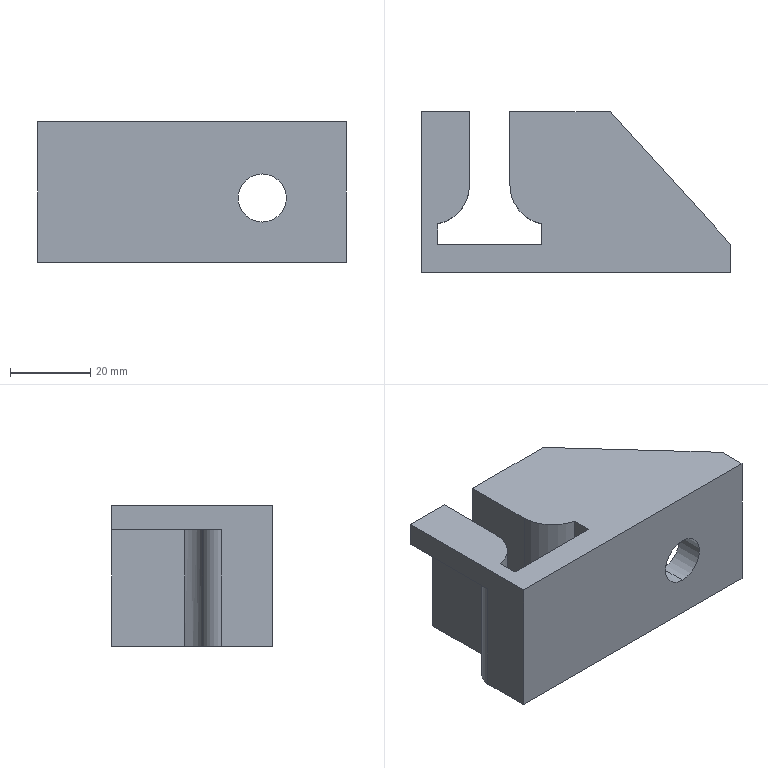Part | SolidWorks | features ICE 4, Fillet 2, MirrorPattern 2, Extrusion 1 | 1 solid | 27 faces | box 77 x 40 x 35 mm | volume 36799 mm3 | plane 19 | cylinder 6 | spline 2 | commonest cylinder face diameters 10 x2 12 x2 20 x2
STEP:
#1=CARTESIAN_POINT('',(39.,0.,-4.638));
#2=VERTEX_POINT('',#1);
#3=CARTESIAN_POINT('',(39.,0.,-16.638));
#4=VERTEX_POINT('',#3);
#5=CARTESIAN_POINT('',(39.,0.,-10.638));
#6=DIRECTION('',(0.,-1.,0.));
#7=DIRECTION('',(0.,0.,1.));
#8=AXIS2_PLACEMENT_3D('',#5,#6,#7);
#9=CIRCLE('',#8,6.);
#10=EDGE_CURVE('',#2,#4,#9,.T.);
#11=ORIENTED_EDGE('',*,*,#10,.T.);
#12=CARTESIAN_POINT('',(39.,7.,-16.638));
#13=VERTEX_POINT('',#12);
#14=CARTESIAN_POINT('',(39.,-3.,-16.638));
#15=DIRECTION('',(0.,1.,0.));
#16=VECTOR('',#15,1000.);
#17=LINE('',#14,#16);
#18=EDGE_CURVE('',#4,#13,#17,.T.);
#19=ORIENTED_EDGE('',*,*,#18,.T.);
#20=CARTESIAN_POINT('',(39.,7.,-4.638));
#21=VERTEX_POINT('',#20);
#22=CARTESIAN_POINT('',(39.,7.,-10.638));
#23=DIRECTION('',(0.,-1.,0.));
#24=DIRECTION('',(0.,0.,1.));
#25=AXIS2_PLACEMENT_3D('',#22,#23,#24);
#26=CIRCLE('',#25,6.);
#27=EDGE_CURVE('',#21,#13,#26,.T.);
#28=ORIENTED_EDGE('',*,*,#27,.F.);
#29=CARTESIAN_POINT('',(39.,-3.,-4.638));
#30=DIRECTION('',(0.,1.,0.));
#31=VECTOR('',#30,1000.);
#32=LINE('',#29,#31);
#33=EDGE_CURVE('',#2,#21,#32,.T.);
#34=ORIENTED_EDGE('',*,*,#33,.F.);
#35=EDGE_LOOP('',(#11,#19,#28,#34));
#36=FACE_OUTER_BOUND('',#35,.T.);
#37=CARTESIAN_POINT('',(39.,-3.,-10.638));
#38=DIRECTION('',(0.,1.,0.));
#39=DIRECTION('',(0.,0.,1.));
#40=AXIS2_PLACEMENT_3D('',#37,#38,#39);
#41=CYLINDRICAL_SURFACE('',#40,6.);
#42=ADVANCED_FACE('',(#36),#41,.F.);
#43=CARTESIAN_POINT('',(17.,7.,-26.638));
#44=VERTEX_POINT('',#43);
#45=CARTESIAN_POINT('',(17.,7.,2.362));
#46=VERTEX_POINT('',#45);
#47=CARTESIAN_POINT('',(17.,7.,-61.752));
#48=DIRECTION('',(0.,0.,1.));
#49=VECTOR('',#48,1000.);
#50=LINE('',#47,#49);
#51=EDGE_CURVE('',#44,#46,#50,.T.);
#52=ORIENTED_EDGE('',*,*,#51,.T.);
#53=CARTESIAN_POINT('',(60.,7.,2.362));
#54=VERTEX_POINT('',#53);
#55=CARTESIAN_POINT('',(13.,7.,2.362));
#56=DIRECTION('',(-1.,0.,0.));
#57=VECTOR('',#56,1000.);
#58=LINE('',#55,#57);
#59=EDGE_CURVE('',#54,#46,#58,.T.);
#60=ORIENTED_EDGE('',*,*,#59,.F.);
#61=CARTESIAN_POINT('',(60.,7.,-26.638));
#62=VERTEX_POINT('',#61);
#63=CARTESIAN_POINT('',(60.,7.,-26.638));
#64=DIRECTION('',(0.,0.,-1.));
#65=VECTOR('',#64,1000.);
#66=LINE('',#63,#65);
#67=EDGE_CURVE('',#54,#62,#66,.T.);
#68=ORIENTED_EDGE('',*,*,#67,.T.);
#69=CARTESIAN_POINT('',(-60.,7.,-26.638));
#70=DIRECTION('',(-1.,0.,0.));
#71=VECTOR('',#70,1000.);
#72=LINE('',#69,#71);
#73=EDGE_CURVE('',#62,#44,#72,.T.);
#74=ORIENTED_EDGE('',*,*,#73,.T.);
#75=EDGE_LOOP('',(#52,#60,#68,#74));
#76=FACE_OUTER_BOUND('',#75,.T.);
#77=ORIENTED_EDGE('',*,*,#27,.T.);
#78=CARTESIAN_POINT('',(39.,7.,-10.638));
#79=DIRECTION('',(0.,-1.,0.));
#80=DIRECTION('',(0.,0.,1.));
#81=AXIS2_PLACEMENT_3D('',#78,#79,#80);
#82=CIRCLE('',#81,6.);
#83=EDGE_CURVE('',#13,#21,#82,.T.);
#84=ORIENTED_EDGE('',*,*,#83,.T.);
#85=EDGE_LOOP('',(#77,#84));
#86=FACE_BOUND('',#85,.T.);
#87=CARTESIAN_POINT('',(0.,7.,0.));
#88=DIRECTION('',(0.,1.,0.));
#89=DIRECTION('',(0.,0.,1.));
#90=AXIS2_PLACEMENT_3D('',#87,#88,#89);
#91=PLANE('',#90);
#92=ADVANCED_FACE('',(#76,#86),#91,.T.);
#93=CARTESIAN_POINT('',(-17.,0.,8.362));
#94=VERTEX_POINT('',#93);
#95=CARTESIAN_POINT('',(60.,0.,8.362));
#96=VERTEX_POINT('',#95);
#97=CARTESIAN_POINT('',(-60.,0.,8.362));
#98=DIRECTION('',(1.,0.,0.));
#99=VECTOR('',#98,1000.);
#100=LINE('',#97,#99);
#101=EDGE_CURVE('',#94,#96,#100,.T.);
#102=ORIENTED_EDGE('',*,*,#101,.F.);
#103=CARTESIAN_POINT('',(-17.,0.,-26.638));
#104=VERTEX_POINT('',#103);
#105=CARTESIAN_POINT('',(-17.,0.,0.));
#106=DIRECTION('',(0.,0.,-1.));
#107=VECTOR('',#106,1000.);
#108=LINE('',#105,#107);
#109=EDGE_CURVE('',#94,#104,#108,.T.);
#110=ORIENTED_EDGE('',*,*,#109,.T.);
#111=CARTESIAN_POINT('',(60.,0.,-26.638));
#112=VERTEX_POINT('',#111);
#113=CARTESIAN_POINT('',(-60.,0.,-26.638));
#114=DIRECTION('',(-1.,0.,0.));
#115=VECTOR('',#114,1000.);
#116=LINE('',#113,#115);
#117=EDGE_CURVE('',#112,#104,#116,.T.);
#118=ORIENTED_EDGE('',*,*,#117,.F.);
#119=CARTESIAN_POINT('',(60.,0.,-26.638));
#120=DIRECTION('',(0.,0.,-1.));
#121=VECTOR('',#120,1000.);
#122=LINE('',#119,#121);
#123=EDGE_CURVE('',#96,#112,#122,.T.);
#124=ORIENTED_EDGE('',*,*,#123,.F.);
#125=EDGE_LOOP('',(#102,#110,#118,#124));
#126=FACE_OUTER_BOUND('',#125,.T.);
#127=ORIENTED_EDGE('',*,*,#10,.F.);
#128=CARTESIAN_POINT('',(39.,0.,-10.638));
#129=DIRECTION('',(0.,-1.,0.));
#130=DIRECTION('',(0.,0.,1.));
#131=AXIS2_PLACEMENT_3D('',#128,#129,#130);
#132=CIRCLE('',#131,6.);
#133=EDGE_CURVE('',#4,#2,#132,.T.);
#134=ORIENTED_EDGE('',*,*,#133,.F.);
#135=EDGE_LOOP('',(#127,#134));
#136=FACE_BOUND('',#135,.T.);
#137=CARTESIAN_POINT('',(0.,0.,0.));
#138=DIRECTION('',(0.,1.,0.));
#139=DIRECTION('',(0.,0.,1.));
#140=AXIS2_PLACEMENT_3D('',#137,#138,#139);
#141=PLANE('',#140);
#142=ADVANCED_FACE('',(#126,#136),#141,.F.);
#143=CARTESIAN_POINT('',(13.,7.,-26.638));
#144=VERTEX_POINT('',#143);
#145=CARTESIAN_POINT('',(13.,7.,8.362));
#146=VERTEX_POINT('',#145);
#147=CARTESIAN_POINT('',(13.,7.,2.362));
#148=DIRECTION('',(0.,0.,1.));
#149=VECTOR('',#148,1000.);
#150=LINE('',#147,#149);
#151=EDGE_CURVE('',#144,#146,#150,.T.);
#152=ORIENTED_EDGE('',*,*,#151,.F.);
#153=CARTESIAN_POINT('',(-13.,7.,-26.638));
#154=VERTEX_POINT('',#153);
#155=CARTESIAN_POINT('',(-60.,7.,-26.638));
#156=DIRECTION('',(-1.,0.,0.));
#157=VECTOR('',#156,1000.);
#158=LINE('',#155,#157);
#159=EDGE_CURVE('',#144,#154,#158,.T.);
#160=ORIENTED_EDGE('',*,*,#159,.T.);
#161=CARTESIAN_POINT('',(-13.,7.,8.362));
#162=VERTEX_POINT('',#161);
#163=CARTESIAN_POINT('',(-13.,7.,2.362));
#164=DIRECTION('',(0.,0.,1.));
#165=VECTOR('',#164,1000.);
#166=LINE('',#163,#165);
#167=EDGE_CURVE('',#154,#162,#166,.T.);
#168=ORIENTED_EDGE('',*,*,#167,.T.);
#169=CARTESIAN_POINT('',(-60.,7.,8.362));
#170=DIRECTION('',(1.,0.,0.));
#171=VECTOR('',#170,1000.);
#172=LINE('',#169,#171);
#173=EDGE_CURVE('',#162,#146,#172,.T.);
#174=ORIENTED_EDGE('',*,*,#173,.T.);
#175=EDGE_LOOP('',(#152,#160,#168,#174));
#176=FACE_OUTER_BOUND('',#175,.T.);
#177=CARTESIAN_POINT('',(0.,7.,0.));
#178=DIRECTION('',(0.,1.,0.));
#179=DIRECTION('',(0.,0.,1.));
#180=AXIS2_PLACEMENT_3D('',#177,#178,#179);
#181=PLANE('',#180);
#182=ADVANCED_FACE('',(#176),#181,.T.);
#183=CARTESIAN_POINT('',(-13.534,17.332,2.362));
#184=VERTEX_POINT('',#183);
#185=CARTESIAN_POINT('',(-17.,12.573,2.362));
#186=VERTEX_POINT('',#185);
#187=CARTESIAN_POINT('',(-12.,12.573,2.362));
#188=DIRECTION('',(0.,0.,1.));
#189=DIRECTION('',(1.,0.,0.));
#190=AXIS2_PLACEMENT_3D('',#187,#188,#189);
#191=CIRCLE('',#190,5.);
#192=EDGE_CURVE('',#184,#186,#191,.T.);
#193=ORIENTED_EDGE('',*,*,#192,.T.);
#194=CARTESIAN_POINT('',(-17.,40.,2.362));
#195=VERTEX_POINT('',#194);
#196=CARTESIAN_POINT('',(-17.,0.,2.362));
#197=DIRECTION('',(0.,1.,0.));
#198=VECTOR('',#197,1000.);
#199=LINE('',#196,#198);
#200=EDGE_CURVE('',#186,#195,#199,.T.);
#201=ORIENTED_EDGE('',*,*,#200,.T.);
#202=CARTESIAN_POINT('',(-9.,40.,2.362));
#203=VERTEX_POINT('',#202);
#204=CARTESIAN_POINT('',(-30.,40.,2.362));
#205=DIRECTION('',(-1.,0.,0.));
#206=VECTOR('',#205,1000.);
#207=LINE('',#204,#206);
#208=EDGE_CURVE('',#203,#195,#207,.T.);
#209=ORIENTED_EDGE('',*,*,#208,.F.);
#210=CARTESIAN_POINT('',(-9.,21.798,2.362));
#211=VERTEX_POINT('',#210);
#212=CARTESIAN_POINT('',(-9.,21.798,2.362));
#213=DIRECTION('',(0.,1.,0.));
#214=VECTOR('',#213,1000.);
#215=LINE('',#212,#214);
#216=EDGE_CURVE('',#211,#203,#215,.T.);
#217=ORIENTED_EDGE('',*,*,#216,.F.);
#218=CARTESIAN_POINT('',(-13.534,17.332,2.362));
#219=CARTESIAN_POINT('',(-10.568,18.288,2.362));
#220=CARTESIAN_POINT('',(-9.,21.798,2.362));
#221=B_SPLINE_CURVE_WITH_KNOTS('',2,(#218,#219,#220),.UNSPECIFIED.,.F.,.F.,(3,3),(0.3423,1.),.UNSPECIFIED.);
#222=EDGE_CURVE('',#184,#211,#221,.T.);
#223=ORIENTED_EDGE('',*,*,#222,.F.);
#224=EDGE_LOOP('',(#193,#201,#209,#217,#223));
#225=FACE_OUTER_BOUND('',#224,.T.);
#226=CARTESIAN_POINT('',(0.,0.,2.362));
#227=DIRECTION('',(0.,0.,1.));
#228=DIRECTION('',(1.,0.,0.));
#229=AXIS2_PLACEMENT_3D('',#226,#227,#228);
#230=PLANE('',#229);
#231=ADVANCED_FACE('',(#225),#230,.F.);
#232=CARTESIAN_POINT('',(-5.,40.,8.362));
#233=VERTEX_POINT('',#232);
#234=CARTESIAN_POINT('',(-17.,40.,8.362));
#235=VERTEX_POINT('',#234);
#236=CARTESIAN_POINT('',(-30.,40.,8.362));
#237=DIRECTION('',(-1.,0.,0.));
#238=VECTOR('',#237,1000.);
#239=LINE('',#236,#238);
#240=EDGE_CURVE('',#233,#235,#239,.T.);
#241=ORIENTED_EDGE('',*,*,#240,.T.);
#242=CARTESIAN_POINT('',(-17.,7.,8.362));
#243=DIRECTION('',(0.,-1.,0.));
#244=VECTOR('',#243,1000.);
#245=LINE('',#242,#244);
#246=EDGE_CURVE('',#235,#94,#245,.T.);
#247=ORIENTED_EDGE('',*,*,#246,.T.);
#248=ORIENTED_EDGE('',*,*,#101,.T.);
#249=CARTESIAN_POINT('',(60.,7.,8.362));
#250=VERTEX_POINT('',#249);
#251=CARTESIAN_POINT('',(60.,7.,8.362));
#252=DIRECTION('',(0.,-1.,0.));
#253=VECTOR('',#252,1000.);
#254=LINE('',#251,#253);
#255=EDGE_CURVE('',#250,#96,#254,.T.);
#256=ORIENTED_EDGE('',*,*,#255,.F.);
#257=CARTESIAN_POINT('',(30.,40.,8.362));
#258=VERTEX_POINT('',#257);
#259=CARTESIAN_POINT('',(60.,7.,8.362));
#260=DIRECTION('',(0.6727,-0.7399,0.));
#261=VECTOR('',#260,1000.);
#262=LINE('',#259,#261);
#263=EDGE_CURVE('',#258,#250,#262,.T.);
#264=ORIENTED_EDGE('',*,*,#263,.F.);
#265=CARTESIAN_POINT('',(5.,40.,8.362));
#266=VERTEX_POINT('',#265);
#267=CARTESIAN_POINT('',(30.,40.,8.362));
#268=DIRECTION('',(1.,0.,0.));
#269=VECTOR('',#268,1000.);
#270=LINE('',#267,#269);
#271=EDGE_CURVE('',#266,#258,#270,.T.);
#272=ORIENTED_EDGE('',*,*,#271,.F.);
#273=CARTESIAN_POINT('',(5.,21.798,8.362));
#274=VERTEX_POINT('',#273);
#275=CARTESIAN_POINT('',(5.,40.,8.362));
#276=DIRECTION('',(0.,1.,0.));
#277=VECTOR('',#276,1000.);
#278=LINE('',#275,#277);
#279=EDGE_CURVE('',#274,#266,#278,.T.);
#280=ORIENTED_EDGE('',*,*,#279,.F.);
#281=CARTESIAN_POINT('',(13.,12.,8.362));
#282=VERTEX_POINT('',#281);
#283=CARTESIAN_POINT('',(15.,21.798,8.362));
#284=DIRECTION('',(0.,0.,1.));
#285=DIRECTION('',(-1.,0.,0.));
#286=AXIS2_PLACEMENT_3D('',#283,#284,#285);
#287=CIRCLE('',#286,10.);
#288=EDGE_CURVE('',#274,#282,#287,.T.);
#289=ORIENTED_EDGE('',*,*,#288,.T.);
#290=CARTESIAN_POINT('',(13.,12.,8.362));
#291=DIRECTION('',(0.,1.,0.));
#292=VECTOR('',#291,1000.);
#293=LINE('',#290,#292);
#294=EDGE_CURVE('',#146,#282,#293,.T.);
#295=ORIENTED_EDGE('',*,*,#294,.F.);
#296=ORIENTED_EDGE('',*,*,#173,.F.);
#297=CARTESIAN_POINT('',(-13.,12.,8.362));
#298=VERTEX_POINT('',#297);
#299=CARTESIAN_POINT('',(-13.,12.,8.362));
#300=DIRECTION('',(0.,1.,0.));
#301=VECTOR('',#300,1000.);
#302=LINE('',#299,#301);
#303=EDGE_CURVE('',#162,#298,#302,.T.);
#304=ORIENTED_EDGE('',*,*,#303,.T.);
#305=CARTESIAN_POINT('',(-5.,21.798,8.362));
#306=VERTEX_POINT('',#305);
#307=CARTESIAN_POINT('',(-15.,21.798,8.362));
#308=DIRECTION('',(0.,0.,1.));
#309=DIRECTION('',(-1.,0.,0.));
#310=AXIS2_PLACEMENT_3D('',#307,#308,#309);
#311=CIRCLE('',#310,10.);
#312=EDGE_CURVE('',#298,#306,#311,.T.);
#313=ORIENTED_EDGE('',*,*,#312,.T.);
#314=CARTESIAN_POINT('',(-5.,40.,8.362));
#315=DIRECTION('',(0.,1.,0.));
#316=VECTOR('',#315,1000.);
#317=LINE('',#314,#316);
#318=EDGE_CURVE('',#306,#233,#317,.T.);
#319=ORIENTED_EDGE('',*,*,#318,.T.);
#320=EDGE_LOOP('',(#241,#247,#248,#256,#264,#272,#280,#289,#295,#296,#304,#313,#319));
#321=FACE_OUTER_BOUND('',#320,.T.);
#322=CARTESIAN_POINT('',(-60.,7.,8.362));
#323=DIRECTION('',(0.,0.,-1.));
#324=DIRECTION('',(-1.,0.,0.));
#325=AXIS2_PLACEMENT_3D('',#322,#323,#324);
#326=PLANE('',#325);
#327=ADVANCED_FACE('',(#321),#326,.F.);
#328=ORIENTED_EDGE('',*,*,#123,.T.);
#329=CARTESIAN_POINT('',(60.,7.,-26.638));
#330=DIRECTION('',(0.,-1.,0.));
#331=VECTOR('',#330,1000.);
#332=LINE('',#329,#331);
#333=EDGE_CURVE('',#62,#112,#332,.T.);
#334=ORIENTED_EDGE('',*,*,#333,.F.);
#335=ORIENTED_EDGE('',*,*,#67,.F.);
#336=CARTESIAN_POINT('',(60.,7.,-26.638));
#337=DIRECTION('',(0.,0.,-1.));
#338=VECTOR('',#337,1000.);
#339=LINE('',#336,#338);
#340=EDGE_CURVE('',#250,#54,#339,.T.);
#341=ORIENTED_EDGE('',*,*,#340,.F.);
#342=ORIENTED_EDGE('',*,*,#255,.T.);
#343=EDGE_LOOP('',(#328,#334,#335,#341,#342));
#344=FACE_OUTER_BOUND('',#343,.T.);
#345=CARTESIAN_POINT('',(60.,7.,-26.638));
#346=DIRECTION('',(-1.,0.,0.));
#347=DIRECTION('',(0.,0.,1.));
#348=AXIS2_PLACEMENT_3D('',#345,#346,#347);
#349=PLANE('',#348);
#350=ADVANCED_FACE('',(#344),#349,.F.);
#351=ORIENTED_EDGE('',*,*,#117,.T.);
#352=CARTESIAN_POINT('',(-17.,12.573,-26.638));
#353=VERTEX_POINT('',#352);
#354=CARTESIAN_POINT('',(-17.,15.,-26.638));
#355=DIRECTION('',(0.,-1.,0.));
#356=VECTOR('',#355,1000.);
#357=LINE('',#354,#356);
#358=EDGE_CURVE('',#353,#104,#357,.T.);
#359=ORIENTED_EDGE('',*,*,#358,.F.);
#360=CARTESIAN_POINT('',(-13.534,17.332,-26.638));
#361=VERTEX_POINT('',#360);
#362=CARTESIAN_POINT('',(-12.,12.573,-26.638));
#363=DIRECTION('',(0.,0.,-1.));
#364=DIRECTION('',(1.,0.,0.));
#365=AXIS2_PLACEMENT_3D('',#362,#363,#364);
#366=CIRCLE('',#365,5.);
#367=EDGE_CURVE('',#353,#361,#366,.T.);
#368=ORIENTED_EDGE('',*,*,#367,.T.);
#369=CARTESIAN_POINT('',(-9.,21.798,-26.638));
#370=VERTEX_POINT('',#369);
#371=CARTESIAN_POINT('',(-9.,21.798,-26.638));
#372=CARTESIAN_POINT('',(-10.568,18.288,-26.638));
#373=CARTESIAN_POINT('',(-13.534,17.332,-26.638));
#374=B_SPLINE_CURVE_WITH_KNOTS('',2,(#371,#372,#373),.UNSPECIFIED.,.F.,.F.,(3,3),(0.,0.6577),.UNSPECIFIED.);
#375=EDGE_CURVE('',#370,#361,#374,.T.);
#376=ORIENTED_EDGE('',*,*,#375,.F.);
#377=CARTESIAN_POINT('',(-9.,40.,-26.638));
#378=VERTEX_POINT('',#377);
#379=CARTESIAN_POINT('',(-9.,21.798,-26.638));
#380=DIRECTION('',(0.,-1.,0.));
#381=VECTOR('',#380,1000.);
#382=LINE('',#379,#381);
#383=EDGE_CURVE('',#378,#370,#382,.T.);
#384=ORIENTED_EDGE('',*,*,#383,.F.);
#385=CARTESIAN_POINT('',(-5.,40.,-26.638));
#386=VERTEX_POINT('',#385);
#387=CARTESIAN_POINT('',(-5.,40.,-26.638));
#388=DIRECTION('',(-1.,0.,0.));
#389=VECTOR('',#388,1000.);
#390=LINE('',#387,#389);
#391=EDGE_CURVE('',#386,#378,#390,.T.);
#392=ORIENTED_EDGE('',*,*,#391,.F.);
#393=CARTESIAN_POINT('',(-5.,21.798,-26.638));
#394=VERTEX_POINT('',#393);
#395=CARTESIAN_POINT('',(-5.,21.798,-26.638));
#396=DIRECTION('',(0.,1.,0.));
#397=VECTOR('',#396,1000.);
#398=LINE('',#395,#397);
#399=EDGE_CURVE('',#394,#386,#398,.T.);
#400=ORIENTED_EDGE('',*,*,#399,.F.);
#401=CARTESIAN_POINT('',(-13.,12.,-26.638));
#402=VERTEX_POINT('',#401);
#403=CARTESIAN_POINT('',(-15.,21.798,-26.638));
#404=DIRECTION('',(0.,0.,1.));
#405=DIRECTION('',(1.,0.,0.));
#406=AXIS2_PLACEMENT_3D('',#403,#404,#405);
#407=CIRCLE('',#406,10.);
#408=EDGE_CURVE('',#402,#394,#407,.T.);
#409=ORIENTED_EDGE('',*,*,#408,.F.);
#410=CARTESIAN_POINT('',(-13.,7.,-26.638));
#411=DIRECTION('',(0.,1.,0.));
#412=VECTOR('',#411,1000.);
#413=LINE('',#410,#412);
#414=EDGE_CURVE('',#154,#402,#413,.T.);
#415=ORIENTED_EDGE('',*,*,#414,.F.);
#416=ORIENTED_EDGE('',*,*,#159,.F.);
#417=CARTESIAN_POINT('',(13.,12.,-26.638));
#418=VERTEX_POINT('',#417);
#419=CARTESIAN_POINT('',(13.,7.,-26.638));
#420=DIRECTION('',(0.,1.,0.));
#421=VECTOR('',#420,1000.);
#422=LINE('',#419,#421);
#423=EDGE_CURVE('',#144,#418,#422,.T.);
#424=ORIENTED_EDGE('',*,*,#423,.T.);
#425=CARTESIAN_POINT('',(5.,21.798,-26.638));
#426=VERTEX_POINT('',#425);
#427=CARTESIAN_POINT('',(15.,21.798,-26.638));
#428=DIRECTION('',(0.,0.,-1.));
#429=DIRECTION('',(1.,0.,0.));
#430=AXIS2_PLACEMENT_3D('',#427,#428,#429);
#431=CIRCLE('',#430,10.);
#432=EDGE_CURVE('',#418,#426,#431,.T.);
#433=ORIENTED_EDGE('',*,*,#432,.T.);
#434=CARTESIAN_POINT('',(5.,40.,-26.638));
#435=VERTEX_POINT('',#434);
#436=CARTESIAN_POINT('',(5.,21.798,-26.638));
#437=DIRECTION('',(0.,1.,0.));
#438=VECTOR('',#437,1000.);
#439=LINE('',#436,#438);
#440=EDGE_CURVE('',#426,#435,#439,.T.);
#441=ORIENTED_EDGE('',*,*,#440,.T.);
#442=CARTESIAN_POINT('',(9.,40.,-26.638));
#443=VERTEX_POINT('',#442);
#444=CARTESIAN_POINT('',(5.,40.,-26.638));
#445=DIRECTION('',(1.,0.,0.));
#446=VECTOR('',#445,1000.);
#447=LINE('',#444,#446);
#448=EDGE_CURVE('',#435,#443,#447,.T.);
#449=ORIENTED_EDGE('',*,*,#448,.T.);
#450=CARTESIAN_POINT('',(9.,21.798,-26.638));
#451=VERTEX_POINT('',#450);
#452=CARTESIAN_POINT('',(9.,21.798,-26.638));
#453=DIRECTION('',(0.,-1.,0.));
#454=VECTOR('',#453,1000.);
#455=LINE('',#452,#454);
#456=EDGE_CURVE('',#443,#451,#455,.T.);
#457=ORIENTED_EDGE('',*,*,#456,.T.);
#458=CARTESIAN_POINT('',(13.534,17.332,-26.638));
#459=VERTEX_POINT('',#458);
#460=CARTESIAN_POINT('',(9.,21.798,-26.638));
#461=CARTESIAN_POINT('',(10.568,18.288,-26.638));
#462=CARTESIAN_POINT('',(13.534,17.332,-26.638));
#463=B_SPLINE_CURVE_WITH_KNOTS('',2,(#460,#461,#462),.UNSPECIFIED.,.F.,.F.,(3,3),(0.,0.6577),.UNSPECIFIED.);
#464=EDGE_CURVE('',#451,#459,#463,.T.);
#465=ORIENTED_EDGE('',*,*,#464,.T.);
#466=CARTESIAN_POINT('',(17.,12.573,-26.638));
#467=VERTEX_POINT('',#466);
#468=CARTESIAN_POINT('',(12.,12.573,-26.638));
#469=DIRECTION('',(0.,0.,-1.));
#470=DIRECTION('',(1.,0.,0.));
#471=AXIS2_PLACEMENT_3D('',#468,#469,#470);
#472=CIRCLE('',#471,5.);
#473=EDGE_CURVE('',#459,#467,#472,.T.);
#474=ORIENTED_EDGE('',*,*,#473,.T.);
#475=CARTESIAN_POINT('',(17.,7.,-26.638));
#476=DIRECTION('',(0.,-1.,0.));
#477=VECTOR('',#476,1000.);
#478=LINE('',#475,#477);
#479=EDGE_CURVE('',#467,#44,#478,.T.);
#480=ORIENTED_EDGE('',*,*,#479,.T.);
#481=ORIENTED_EDGE('',*,*,#73,.F.);
#482=ORIENTED_EDGE('',*,*,#333,.T.);
#483=EDGE_LOOP('',(#351,#359,#368,#376,#384,#392,#400,#409,#415,#416,#424,#433,#441,#449,#457,#465,#474,#480,#481,#482));
#484=FACE_OUTER_BOUND('',#483,.T.);
#485=CARTESIAN_POINT('',(-60.,7.,-26.638));
#486=DIRECTION('',(0.,0.,1.));
#487=DIRECTION('',(1.,0.,0.));
#488=AXIS2_PLACEMENT_3D('',#485,#486,#487);
#489=PLANE('',#488);
#490=ADVANCED_FACE('',(#484),#489,.F.);
#491=CARTESIAN_POINT('',(-17.,40.,2.362));
#492=DIRECTION('',(0.,0.,-1.));
#493=VECTOR('',#492,1000.);
#494=LINE('',#491,#493);
#495=EDGE_CURVE('',#235,#195,#494,.T.);
#496=ORIENTED_EDGE('',*,*,#495,.F.);
#497=ORIENTED_EDGE('',*,*,#240,.F.);
#498=CARTESIAN_POINT('',(-5.,40.,2.362));
#499=DIRECTION('',(0.,0.,1.));
#500=VECTOR('',#499,1000.);
#501=LINE('',#498,#500);
#502=EDGE_CURVE('',#386,#233,#501,.T.);
#503=ORIENTED_EDGE('',*,*,#502,.F.);
#504=ORIENTED_EDGE('',*,*,#391,.T.);
#505=CARTESIAN_POINT('',(-9.,40.,-61.752));
#506=DIRECTION('',(0.,0.,1.));
#507=VECTOR('',#506,1000.);
#508=LINE('',#505,#507);
#509=EDGE_CURVE('',#378,#203,#508,.T.);
#510=ORIENTED_EDGE('',*,*,#509,.T.);
#511=ORIENTED_EDGE('',*,*,#208,.T.);
#512=EDGE_LOOP('',(#496,#497,#503,#504,#510,#511));
#513=FACE_OUTER_BOUND('',#512,.T.);
#514=CARTESIAN_POINT('',(-30.,40.,2.362));
#515=DIRECTION('',(0.,1.,0.));
#516=DIRECTION('',(-1.,0.,0.));
#517=AXIS2_PLACEMENT_3D('',#514,#515,#516);
#518=PLANE('',#517);
#519=ADVANCED_FACE('',(#513),#518,.T.);
#520=ORIENTED_EDGE('',*,*,#318,.F.);
#521=CARTESIAN_POINT('',(-5.,21.798,2.362));
#522=DIRECTION('',(0.,0.,-1.));
#523=VECTOR('',#522,1000.);
#524=LINE('',#521,#523);
#525=EDGE_CURVE('',#306,#394,#524,.T.);
#526=ORIENTED_EDGE('',*,*,#525,.T.);
#527=ORIENTED_EDGE('',*,*,#399,.T.);
#528=ORIENTED_EDGE('',*,*,#502,.T.);
#529=EDGE_LOOP('',(#520,#526,#527,#528));
#530=FACE_OUTER_BOUND('',#529,.T.);
#531=CARTESIAN_POINT('',(-5.,40.,2.362));
#532=DIRECTION('',(1.,0.,0.));
#533=DIRECTION('',(0.,1.,0.));
#534=AXIS2_PLACEMENT_3D('',#531,#532,#533);
#535=PLANE('',#534);
#536=ADVANCED_FACE('',(#530),#535,.T.);
#537=ORIENTED_EDGE('',*,*,#303,.F.);
#538=ORIENTED_EDGE('',*,*,#167,.F.);
#539=ORIENTED_EDGE('',*,*,#414,.T.);
#540=CARTESIAN_POINT('',(-13.,12.,2.362));
#541=DIRECTION('',(0.,0.,1.));
#542=VECTOR('',#541,1000.);
#543=LINE('',#540,#542);
#544=EDGE_CURVE('',#402,#298,#543,.T.);
#545=ORIENTED_EDGE('',*,*,#544,.T.);
#546=EDGE_LOOP('',(#537,#538,#539,#545));
#547=FACE_OUTER_BOUND('',#546,.T.);
#548=CARTESIAN_POINT('',(-13.,12.,2.362));
#549=DIRECTION('',(1.,0.,0.));
#550=DIRECTION('',(0.,1.,0.));
#551=AXIS2_PLACEMENT_3D('',#548,#549,#550);
#552=PLANE('',#551);
#553=ADVANCED_FACE('',(#547),#552,.T.);
#554=ORIENTED_EDGE('',*,*,#544,.F.);
#555=ORIENTED_EDGE('',*,*,#408,.T.);
#556=ORIENTED_EDGE('',*,*,#525,.F.);
#557=ORIENTED_EDGE('',*,*,#312,.F.);
#558=EDGE_LOOP('',(#554,#555,#556,#557));
#559=FACE_OUTER_BOUND('',#558,.T.);
#560=CARTESIAN_POINT('',(-15.,21.798,2.362));
#561=DIRECTION('',(0.,0.,1.));
#562=DIRECTION('',(1.,0.,0.));
#563=AXIS2_PLACEMENT_3D('',#560,#561,#562);
#564=CYLINDRICAL_SURFACE('',#563,10.);
#565=ADVANCED_FACE('',(#559),#564,.T.);
#566=ORIENTED_EDGE('',*,*,#509,.F.);
#567=ORIENTED_EDGE('',*,*,#383,.T.);
#568=CARTESIAN_POINT('',(-9.,21.798,-61.752));
#569=DIRECTION('',(0.,0.,1.));
#570=VECTOR('',#569,1000.);
#571=LINE('',#568,#570);
#572=EDGE_CURVE('',#370,#211,#571,.T.);
#573=ORIENTED_EDGE('',*,*,#572,.T.);
#574=ORIENTED_EDGE('',*,*,#216,.T.);
#575=EDGE_LOOP('',(#566,#567,#573,#574));
#576=FACE_OUTER_BOUND('',#575,.T.);
#577=CARTESIAN_POINT('',(-9.,21.798,-61.752));
#578=DIRECTION('',(1.,0.,0.));
#579=DIRECTION('',(0.,0.,-1.));
#580=AXIS2_PLACEMENT_3D('',#577,#578,#579);
#581=PLANE('',#580);
#582=ADVANCED_FACE('',(#576),#581,.F.);
#583=ORIENTED_EDGE('',*,*,#375,.T.);
#584=CARTESIAN_POINT('',(-13.534,17.332,-26.638));
#585=DIRECTION('',(0.,0.,1.));
#586=VECTOR('',#585,1000.);
#587=LINE('',#584,#586);
#588=EDGE_CURVE('',#361,#184,#587,.T.);
#589=ORIENTED_EDGE('',*,*,#588,.T.);
#590=ORIENTED_EDGE('',*,*,#222,.T.);
#591=ORIENTED_EDGE('',*,*,#572,.F.);
#592=EDGE_LOOP('',(#583,#589,#590,#591));
#593=FACE_OUTER_BOUND('',#592,.T.);
#594=CARTESIAN_POINT('',(-13.534,17.332,-26.638));
#595=CARTESIAN_POINT('',(-13.534,17.332,2.362));
#596=CARTESIAN_POINT('',(-10.568,18.288,-26.638));
#597=CARTESIAN_POINT('',(-10.568,18.288,2.362));
#598=CARTESIAN_POINT('',(-9.,21.798,-26.638));
#599=CARTESIAN_POINT('',(-9.,21.798,2.362));
#600=B_SPLINE_SURFACE_WITH_KNOTS('',2,1,((#594,#595),(#596,#597),(#598,#599)),.UNSPECIFIED.,.F.,.F.,.F.,(3,3),(2,2),(0.3423,1.),(0.,1.),.UNSPECIFIED.);
#601=ADVANCED_FACE('',(#593),#600,.F.);
#602=ORIENTED_EDGE('',*,*,#358,.T.);
#603=ORIENTED_EDGE('',*,*,#109,.F.);
#604=ORIENTED_EDGE('',*,*,#246,.F.);
#605=ORIENTED_EDGE('',*,*,#495,.T.);
#606=ORIENTED_EDGE('',*,*,#200,.F.);
#607=CARTESIAN_POINT('',(-17.,12.573,-61.752));
#608=DIRECTION('',(0.,0.,-1.));
#609=VECTOR('',#608,1000.);
#610=LINE('',#607,#609);
#611=EDGE_CURVE('',#186,#353,#610,.T.);
#612=ORIENTED_EDGE('',*,*,#611,.T.);
#613=EDGE_LOOP('',(#602,#603,#604,#605,#606,#612));
#614=FACE_OUTER_BOUND('',#613,.T.);
#615=CARTESIAN_POINT('',(-17.,15.,-61.752));
#616=DIRECTION('',(1.,0.,0.));
#617=DIRECTION('',(0.,0.,-1.));
#618=AXIS2_PLACEMENT_3D('',#615,#616,#617);
#619=PLANE('',#618);
#620=ADVANCED_FACE('',(#614),#619,.F.);
#621=ORIENTED_EDGE('',*,*,#294,.T.);
#622=CARTESIAN_POINT('',(13.,12.,2.362));
#623=DIRECTION('',(0.,0.,1.));
#624=VECTOR('',#623,1000.);
#625=LINE('',#622,#624);
#626=EDGE_CURVE('',#418,#282,#625,.T.);
#627=ORIENTED_EDGE('',*,*,#626,.F.);
#628=ORIENTED_EDGE('',*,*,#423,.F.);
#629=ORIENTED_EDGE('',*,*,#151,.T.);
#630=EDGE_LOOP('',(#621,#627,#628,#629));
#631=FACE_OUTER_BOUND('',#630,.T.);
#632=CARTESIAN_POINT('',(13.,12.,2.362));
#633=DIRECTION('',(1.,0.,0.));
#634=DIRECTION('',(0.,1.,0.));
#635=AXIS2_PLACEMENT_3D('',#632,#633,#634);
#636=PLANE('',#635);
#637=ADVANCED_FACE('',(#631),#636,.F.);
#638=CARTESIAN_POINT('',(5.,40.,2.362));
#639=DIRECTION('',(0.,0.,1.));
#640=VECTOR('',#639,1000.);
#641=LINE('',#638,#640);
#642=EDGE_CURVE('',#435,#266,#641,.T.);
#643=ORIENTED_EDGE('',*,*,#642,.F.);
#644=ORIENTED_EDGE('',*,*,#440,.F.);
#645=CARTESIAN_POINT('',(5.,21.798,2.362));
#646=DIRECTION('',(0.,0.,1.));
#647=VECTOR('',#646,1000.);
#648=LINE('',#645,#647);
#649=EDGE_CURVE('',#426,#274,#648,.T.);
#650=ORIENTED_EDGE('',*,*,#649,.T.);
#651=ORIENTED_EDGE('',*,*,#279,.T.);
#652=EDGE_LOOP('',(#643,#644,#650,#651));
#653=FACE_OUTER_BOUND('',#652,.T.);
#654=CARTESIAN_POINT('',(5.,40.,2.362));
#655=DIRECTION('',(1.,0.,0.));
#656=DIRECTION('',(0.,1.,0.));
#657=AXIS2_PLACEMENT_3D('',#654,#655,#656);
#658=PLANE('',#657);
#659=ADVANCED_FACE('',(#653),#658,.F.);
#660=ORIENTED_EDGE('',*,*,#271,.T.);
#661=CARTESIAN_POINT('',(30.,40.,2.362));
#662=VERTEX_POINT('',#661);
#663=CARTESIAN_POINT('',(30.,40.,2.362));
#664=DIRECTION('',(0.,0.,1.));
#665=VECTOR('',#664,1000.);
#666=LINE('',#663,#665);
#667=EDGE_CURVE('',#662,#258,#666,.T.);
#668=ORIENTED_EDGE('',*,*,#667,.F.);
#669=CARTESIAN_POINT('',(9.,40.,2.362));
#670=VERTEX_POINT('',#669);
#671=CARTESIAN_POINT('',(30.,40.,2.362));
#672=DIRECTION('',(1.,0.,0.));
#673=VECTOR('',#672,1000.);
#674=LINE('',#671,#673);
#675=EDGE_CURVE('',#670,#662,#674,.T.);
#676=ORIENTED_EDGE('',*,*,#675,.F.);
#677=CARTESIAN_POINT('',(9.,40.,-61.752));
#678=DIRECTION('',(0.,0.,1.));
#679=VECTOR('',#678,1000.);
#680=LINE('',#677,#679);
#681=EDGE_CURVE('',#443,#670,#680,.T.);
#682=ORIENTED_EDGE('',*,*,#681,.F.);
#683=ORIENTED_EDGE('',*,*,#448,.F.);
#684=ORIENTED_EDGE('',*,*,#642,.T.);
#685=EDGE_LOOP('',(#660,#668,#676,#682,#683,#684));
#686=FACE_OUTER_BOUND('',#685,.T.);
#687=CARTESIAN_POINT('',(30.,40.,2.362));
#688=DIRECTION('',(0.,-1.,0.));
#689=DIRECTION('',(1.,0.,0.));
#690=AXIS2_PLACEMENT_3D('',#687,#688,#689);
#691=PLANE('',#690);
#692=ADVANCED_FACE('',(#686),#691,.F.);
#693=ORIENTED_EDGE('',*,*,#263,.T.);
#694=ORIENTED_EDGE('',*,*,#340,.T.);
#695=CARTESIAN_POINT('',(60.,7.,2.362));
#696=DIRECTION('',(0.6727,-0.7399,0.));
#697=VECTOR('',#696,1000.);
#698=LINE('',#695,#697);
#699=EDGE_CURVE('',#662,#54,#698,.T.);
#700=ORIENTED_EDGE('',*,*,#699,.F.);
#701=ORIENTED_EDGE('',*,*,#667,.T.);
#702=EDGE_LOOP('',(#693,#694,#700,#701));
#703=FACE_OUTER_BOUND('',#702,.T.);
#704=CARTESIAN_POINT('',(60.,7.,2.362));
#705=DIRECTION('',(-0.7399,-0.6727,0.));
#706=DIRECTION('',(0.6727,-0.7399,0.));
#707=AXIS2_PLACEMENT_3D('',#704,#705,#706);
#708=PLANE('',#707);
#709=ADVANCED_FACE('',(#703),#708,.F.);
#710=CARTESIAN_POINT('',(17.,12.573,2.362));
#711=VERTEX_POINT('',#710);
#712=CARTESIAN_POINT('',(17.,7.,2.362));
#713=DIRECTION('',(0.,1.,0.));
#714=VECTOR('',#713,1000.);
#715=LINE('',#712,#714);
#716=EDGE_CURVE('',#46,#711,#715,.T.);
#717=ORIENTED_EDGE('',*,*,#716,.T.);
#718=CARTESIAN_POINT('',(13.534,17.332,2.362));
#719=VERTEX_POINT('',#718);
#720=CARTESIAN_POINT('',(12.,12.573,2.362));
#721=DIRECTION('',(0.,0.,1.));
#722=DIRECTION('',(1.,0.,0.));
#723=AXIS2_PLACEMENT_3D('',#720,#721,#722);
#724=CIRCLE('',#723,5.);
#725=EDGE_CURVE('',#711,#719,#724,.T.);
#726=ORIENTED_EDGE('',*,*,#725,.T.);
#727=CARTESIAN_POINT('',(9.,21.798,2.362));
#728=VERTEX_POINT('',#727);
#729=CARTESIAN_POINT('',(13.534,17.332,2.362));
#730=CARTESIAN_POINT('',(10.568,18.288,2.362));
#731=CARTESIAN_POINT('',(9.,21.798,2.362));
#732=B_SPLINE_CURVE_WITH_KNOTS('',2,(#729,#730,#731),.UNSPECIFIED.,.F.,.F.,(3,3),(0.3423,1.),.UNSPECIFIED.);
#733=EDGE_CURVE('',#719,#728,#732,.T.);
#734=ORIENTED_EDGE('',*,*,#733,.T.);
#735=CARTESIAN_POINT('',(9.,21.798,2.362));
#736=DIRECTION('',(0.,1.,0.));
#737=VECTOR('',#736,1000.);
#738=LINE('',#735,#737);
#739=EDGE_CURVE('',#728,#670,#738,.T.);
#740=ORIENTED_EDGE('',*,*,#739,.T.);
#741=ORIENTED_EDGE('',*,*,#675,.T.);
#742=ORIENTED_EDGE('',*,*,#699,.T.);
#743=ORIENTED_EDGE('',*,*,#59,.T.);
#744=EDGE_LOOP('',(#717,#726,#734,#740,#741,#742,#743));
#745=FACE_OUTER_BOUND('',#744,.T.);
#746=CARTESIAN_POINT('',(0.,0.,2.362));
#747=DIRECTION('',(0.,0.,1.));
#748=DIRECTION('',(-1.,0.,0.));
#749=AXIS2_PLACEMENT_3D('',#746,#747,#748);
#750=PLANE('',#749);
#751=ADVANCED_FACE('',(#745),#750,.F.);
#752=ORIENTED_EDGE('',*,*,#649,.F.);
#753=ORIENTED_EDGE('',*,*,#432,.F.);
#754=ORIENTED_EDGE('',*,*,#626,.T.);
#755=ORIENTED_EDGE('',*,*,#288,.F.);
#756=EDGE_LOOP('',(#752,#753,#754,#755));
#757=FACE_OUTER_BOUND('',#756,.T.);
#758=CARTESIAN_POINT('',(15.,21.798,2.362));
#759=DIRECTION('',(0.,0.,-1.));
#760=DIRECTION('',(-1.,0.,0.));
#761=AXIS2_PLACEMENT_3D('',#758,#759,#760);
#762=CYLINDRICAL_SURFACE('',#761,10.);
#763=ADVANCED_FACE('',(#757),#762,.T.);
#764=ORIENTED_EDGE('',*,*,#456,.F.);
#765=ORIENTED_EDGE('',*,*,#681,.T.);
#766=ORIENTED_EDGE('',*,*,#739,.F.);
#767=CARTESIAN_POINT('',(9.,21.798,-61.752));
#768=DIRECTION('',(0.,0.,1.));
#769=VECTOR('',#768,1000.);
#770=LINE('',#767,#769);
#771=EDGE_CURVE('',#451,#728,#770,.T.);
#772=ORIENTED_EDGE('',*,*,#771,.F.);
#773=EDGE_LOOP('',(#764,#765,#766,#772));
#774=FACE_OUTER_BOUND('',#773,.T.);
#775=CARTESIAN_POINT('',(9.,21.798,-61.752));
#776=DIRECTION('',(1.,0.,0.));
#777=DIRECTION('',(0.,0.,-1.));
#778=AXIS2_PLACEMENT_3D('',#775,#776,#777);
#779=PLANE('',#778);
#780=ADVANCED_FACE('',(#774),#779,.T.);
#781=ORIENTED_EDGE('',*,*,#733,.F.);
#782=CARTESIAN_POINT('',(13.534,17.332,2.362));
#783=DIRECTION('',(0.,0.,-1.));
#784=VECTOR('',#783,1000.);
#785=LINE('',#782,#784);
#786=EDGE_CURVE('',#719,#459,#785,.T.);
#787=ORIENTED_EDGE('',*,*,#786,.T.);
#788=ORIENTED_EDGE('',*,*,#464,.F.);
#789=ORIENTED_EDGE('',*,*,#771,.T.);
#790=EDGE_LOOP('',(#781,#787,#788,#789));
#791=FACE_OUTER_BOUND('',#790,.T.);
#792=CARTESIAN_POINT('',(13.534,17.332,-26.638));
#793=CARTESIAN_POINT('',(13.534,17.332,2.362));
#794=CARTESIAN_POINT('',(10.568,18.288,-26.638));
#795=CARTESIAN_POINT('',(10.568,18.288,2.362));
#796=CARTESIAN_POINT('',(9.,21.798,-26.638));
#797=CARTESIAN_POINT('',(9.,21.798,2.362));
#798=B_SPLINE_SURFACE_WITH_KNOTS('',2,1,((#792,#793),(#794,#795),(#796,#797)),.UNSPECIFIED.,.F.,.F.,.F.,(3,3),(2,2),(0.3423,1.),(0.,1.),.UNSPECIFIED.);
#799=ADVANCED_FACE('',(#791),#798,.T.);
#800=ORIENTED_EDGE('',*,*,#479,.F.);
#801=CARTESIAN_POINT('',(17.,12.573,-61.752));
#802=DIRECTION('',(0.,0.,1.));
#803=VECTOR('',#802,1000.);
#804=LINE('',#801,#803);
#805=EDGE_CURVE('',#467,#711,#804,.T.);
#806=ORIENTED_EDGE('',*,*,#805,.T.);
#807=ORIENTED_EDGE('',*,*,#716,.F.);
#808=ORIENTED_EDGE('',*,*,#51,.F.);
#809=EDGE_LOOP('',(#800,#806,#807,#808));
#810=FACE_OUTER_BOUND('',#809,.T.);
#811=CARTESIAN_POINT('',(17.,7.,-61.752));
#812=DIRECTION('',(1.,0.,0.));
#813=DIRECTION('',(0.,0.,-1.));
#814=AXIS2_PLACEMENT_3D('',#811,#812,#813);
#815=PLANE('',#814);
#816=ADVANCED_FACE('',(#810),#815,.T.);
#817=ORIENTED_EDGE('',*,*,#18,.F.);
#818=ORIENTED_EDGE('',*,*,#133,.T.);
#819=ORIENTED_EDGE('',*,*,#33,.T.);
#820=ORIENTED_EDGE('',*,*,#83,.F.);
#821=EDGE_LOOP('',(#817,#818,#819,#820));
#822=FACE_OUTER_BOUND('',#821,.T.);
#823=CARTESIAN_POINT('',(39.,-3.,-10.638));
#824=DIRECTION('',(0.,1.,0.));
#825=DIRECTION('',(0.,0.,1.));
#826=AXIS2_PLACEMENT_3D('',#823,#824,#825);
#827=CYLINDRICAL_SURFACE('',#826,6.);
#828=ADVANCED_FACE('',(#822),#827,.F.);
#829=ORIENTED_EDGE('',*,*,#367,.F.);
#830=ORIENTED_EDGE('',*,*,#611,.F.);
#831=ORIENTED_EDGE('',*,*,#192,.F.);
#832=ORIENTED_EDGE('',*,*,#588,.F.);
#833=EDGE_LOOP('',(#829,#830,#831,#832));
#834=FACE_OUTER_BOUND('',#833,.T.);
#835=CARTESIAN_POINT('',(-12.,12.573,-12.138));
#836=DIRECTION('',(0.,0.,1.));
#837=DIRECTION('',(1.,0.,0.));
#838=AXIS2_PLACEMENT_3D('',#835,#836,#837);
#839=CYLINDRICAL_SURFACE('',#838,5.);
#840=ADVANCED_FACE('',(#834),#839,.T.);
#841=ORIENTED_EDGE('',*,*,#473,.F.);
#842=ORIENTED_EDGE('',*,*,#786,.F.);
#843=ORIENTED_EDGE('',*,*,#725,.F.);
#844=ORIENTED_EDGE('',*,*,#805,.F.);
#845=EDGE_LOOP('',(#841,#842,#843,#844));
#846=FACE_OUTER_BOUND('',#845,.T.);
#847=CARTESIAN_POINT('',(12.,12.573,-12.138));
#848=DIRECTION('',(0.,0.,1.));
#849=DIRECTION('',(1.,0.,0.));
#850=AXIS2_PLACEMENT_3D('',#847,#848,#849);
#851=CYLINDRICAL_SURFACE('',#850,5.);
#852=ADVANCED_FACE('',(#846),#851,.T.);
#853=CLOSED_SHELL('',(#42,#92,#142,#182,#231,#327,#350,#490,#519,#536,#553,#565,#582,#601,#620,#637,#659,#692,#709,#751,#763,#780,#799,#816,#828,#840,#852));
#854=MANIFOLD_SOLID_BREP('',#853);
#855=CARTESIAN_POINT('',(0.,0.,0.));
#856=DIRECTION('',(0.,0.,1.));
#857=DIRECTION('',(1.,0.,0.));
#858=AXIS2_PLACEMENT_3D('',#855,#856,#857);
#859=(LENGTH_UNIT()NAMED_UNIT(*)SI_UNIT(.MILLI.,.METRE.));
#860=UNCERTAINTY_MEASURE_WITH_UNIT(LENGTH_MEASURE(0.00001),#859,'','');
#861=(NAMED_UNIT(*)PLANE_ANGLE_UNIT()SI_UNIT($,.RADIAN.));
#862=(NAMED_UNIT(*)SI_UNIT($,.STERADIAN.)SOLID_ANGLE_UNIT());
#863=(GEOMETRIC_REPRESENTATION_CONTEXT(3)GLOBAL_UNCERTAINTY_ASSIGNED_CONTEXT((#860))GLOBAL_UNIT_ASSIGNED_CONTEXT((#859,#861,#862))REPRESENTATION_CONTEXT('',''));
#864=ADVANCED_BREP_SHAPE_REPRESENTATION('',(#854,#858),#863);